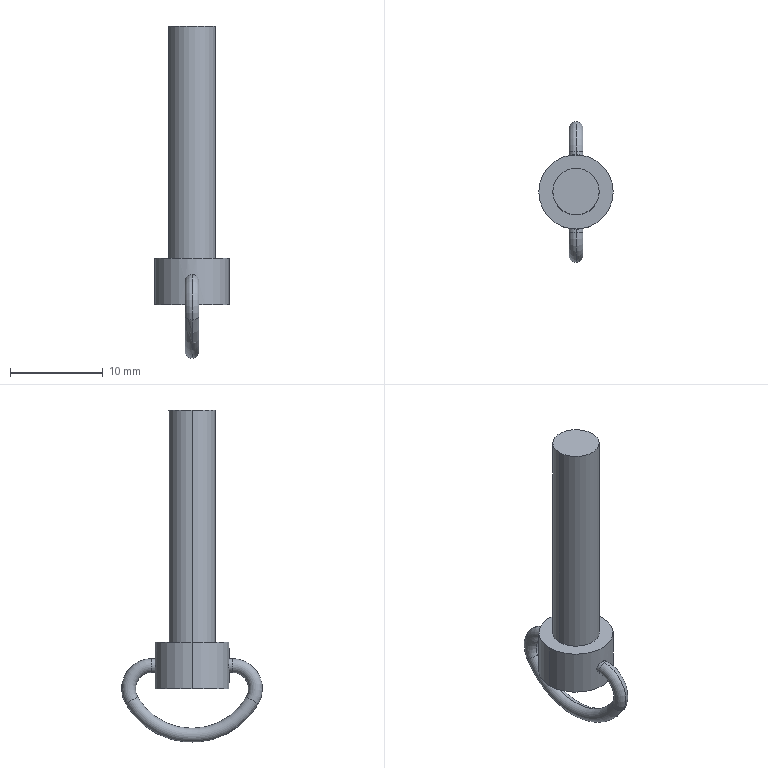Part | SolidWorks | features Extrusion 1, ICE 1, Sweep 1 | 1 solid | 17 faces | box 8 x 15.16 x 35.75 mm | volume 789.697 mm3 | cylinder 8 | torus 6 | plane 3 | commonest cylinder face diameters 1.5 x4 5 x2 8 x2
STEP:
#1=CARTESIAN_POINT('',(0.,4.33,1.75));
#2=VERTEX_POINT('',#1);
#3=CARTESIAN_POINT('',(0.,4.33,3.25));
#4=VERTEX_POINT('',#3);
#5=CARTESIAN_POINT('',(0.,4.33,2.5));
#6=DIRECTION('',(0.,1.,0.));
#7=DIRECTION('',(0.,0.,1.));
#8=AXIS2_PLACEMENT_3D('',#5,#6,#7);
#9=CIRCLE('',#8,0.75);
#10=EDGE_CURVE('',#2,#4,#9,.T.);
#11=ORIENTED_EDGE('',*,*,#10,.T.);
#12=CARTESIAN_POINT('',(0.,7.145,-1.625));
#13=VERTEX_POINT('',#12);
#14=CARTESIAN_POINT('',(0.,4.33,0.));
#15=DIRECTION('',(-1.,0.,0.));
#16=DIRECTION('',(0.,0.,1.));
#17=AXIS2_PLACEMENT_3D('',#14,#15,#16);
#18=CIRCLE('',#17,3.25);
#19=EDGE_CURVE('',#4,#13,#18,.T.);
#20=ORIENTED_EDGE('',*,*,#19,.T.);
#21=CARTESIAN_POINT('',(0.,5.846,-0.875));
#22=VERTEX_POINT('',#21);
#23=CARTESIAN_POINT('',(0.,6.495,-1.25));
#24=DIRECTION('',(0.,-0.5,-0.866));
#25=DIRECTION('',(0.,0.866,-0.5));
#26=AXIS2_PLACEMENT_3D('',#23,#24,#25);
#27=CIRCLE('',#26,0.75);
#28=EDGE_CURVE('',#22,#13,#27,.T.);
#29=ORIENTED_EDGE('',*,*,#28,.F.);
#30=CARTESIAN_POINT('',(0.,4.33,0.));
#31=DIRECTION('',(-1.,0.,0.));
#32=DIRECTION('',(0.,0.,1.));
#33=AXIS2_PLACEMENT_3D('',#30,#31,#32);
#34=CIRCLE('',#33,1.75);
#35=EDGE_CURVE('',#2,#22,#34,.T.);
#36=ORIENTED_EDGE('',*,*,#35,.F.);
#37=EDGE_LOOP('',(#11,#20,#29,#36));
#38=FACE_OUTER_BOUND('',#37,.T.);
#39=CARTESIAN_POINT('',(0.,4.33,0.));
#40=DIRECTION('',(-1.,0.,0.));
#41=DIRECTION('',(0.,0.,1.));
#42=AXIS2_PLACEMENT_3D('',#39,#40,#41);
#43=TOROIDAL_SURFACE('',#42,2.5,0.75);
#44=ADVANCED_FACE('',(#38),#43,.T.);
#45=ORIENTED_EDGE('',*,*,#28,.T.);
#46=CARTESIAN_POINT('',(0.,-7.145,-1.625));
#47=VERTEX_POINT('',#46);
#48=CARTESIAN_POINT('',(0.,0.,2.5));
#49=DIRECTION('',(-1.,0.,0.));
#50=DIRECTION('',(0.,0.,1.));
#51=AXIS2_PLACEMENT_3D('',#48,#49,#50);
#52=CIRCLE('',#51,8.25);
#53=EDGE_CURVE('',#13,#47,#52,.T.);
#54=ORIENTED_EDGE('',*,*,#53,.T.);
#55=CARTESIAN_POINT('',(0.,-5.846,-0.875));
#56=VERTEX_POINT('',#55);
#57=CARTESIAN_POINT('',(0.,-6.495,-1.25));
#58=DIRECTION('',(0.,-0.5,0.866));
#59=DIRECTION('',(0.,-0.866,-0.5));
#60=AXIS2_PLACEMENT_3D('',#57,#58,#59);
#61=CIRCLE('',#60,0.75);
#62=EDGE_CURVE('',#56,#47,#61,.T.);
#63=ORIENTED_EDGE('',*,*,#62,.F.);
#64=CARTESIAN_POINT('',(0.,0.,2.5));
#65=DIRECTION('',(-1.,0.,0.));
#66=DIRECTION('',(0.,0.,1.));
#67=AXIS2_PLACEMENT_3D('',#64,#65,#66);
#68=CIRCLE('',#67,6.75);
#69=EDGE_CURVE('',#22,#56,#68,.T.);
#70=ORIENTED_EDGE('',*,*,#69,.F.);
#71=EDGE_LOOP('',(#45,#54,#63,#70));
#72=FACE_OUTER_BOUND('',#71,.T.);
#73=CARTESIAN_POINT('',(0.,0.,2.5));
#74=DIRECTION('',(-1.,0.,0.));
#75=DIRECTION('',(0.,0.,1.));
#76=AXIS2_PLACEMENT_3D('',#73,#74,#75);
#77=TOROIDAL_SURFACE('',#76,7.5,0.75);
#78=ADVANCED_FACE('',(#72),#77,.T.);
#79=ORIENTED_EDGE('',*,*,#62,.T.);
#80=CARTESIAN_POINT('',(0.,-4.33,3.25));
#81=VERTEX_POINT('',#80);
#82=CARTESIAN_POINT('',(0.,-4.33,0.));
#83=DIRECTION('',(-1.,0.,0.));
#84=DIRECTION('',(0.,0.,1.));
#85=AXIS2_PLACEMENT_3D('',#82,#83,#84);
#86=CIRCLE('',#85,3.25);
#87=EDGE_CURVE('',#47,#81,#86,.T.);
#88=ORIENTED_EDGE('',*,*,#87,.T.);
#89=CARTESIAN_POINT('',(0.,-4.33,1.75));
#90=VERTEX_POINT('',#89);
#91=CARTESIAN_POINT('',(0.,-4.33,2.5));
#92=DIRECTION('',(0.,1.,0.));
#93=DIRECTION('',(0.,0.,1.));
#94=AXIS2_PLACEMENT_3D('',#91,#92,#93);
#95=CIRCLE('',#94,0.75);
#96=EDGE_CURVE('',#90,#81,#95,.T.);
#97=ORIENTED_EDGE('',*,*,#96,.F.);
#98=CARTESIAN_POINT('',(0.,-4.33,0.));
#99=DIRECTION('',(-1.,0.,0.));
#100=DIRECTION('',(0.,0.,1.));
#101=AXIS2_PLACEMENT_3D('',#98,#99,#100);
#102=CIRCLE('',#101,1.75);
#103=EDGE_CURVE('',#56,#90,#102,.T.);
#104=ORIENTED_EDGE('',*,*,#103,.F.);
#105=EDGE_LOOP('',(#79,#88,#97,#104));
#106=FACE_OUTER_BOUND('',#105,.T.);
#107=CARTESIAN_POINT('',(0.,-4.33,0.));
#108=DIRECTION('',(-1.,0.,0.));
#109=DIRECTION('',(0.,0.,1.));
#110=AXIS2_PLACEMENT_3D('',#107,#108,#109);
#111=TOROIDAL_SURFACE('',#110,2.5,0.75);
#112=ADVANCED_FACE('',(#106),#111,.T.);
#113=CARTESIAN_POINT('',(0.,-4.,1.75));
#114=VERTEX_POINT('',#113);
#115=CARTESIAN_POINT('',(0.,-4.,3.25));
#116=VERTEX_POINT('',#115);
#117=CARTESIAN_POINT('',(0.,-4.,1.75));
#118=CARTESIAN_POINT('',(0.09935,-4.,1.75));
#119=CARTESIAN_POINT('',(0.1968,-3.996,1.77));
#120=CARTESIAN_POINT('',(0.3784,-3.983,1.845));
#121=CARTESIAN_POINT('',(0.4614,-3.974,1.901));
#122=CARTESIAN_POINT('',(0.6685,-3.946,2.108));
#123=CARTESIAN_POINT('',(0.7499,-3.929,2.304));
#124=CARTESIAN_POINT('',(0.75,-3.929,2.598));
#125=CARTESIAN_POINT('',(0.7305,-3.933,2.696));
#126=CARTESIAN_POINT('',(0.6552,-3.946,2.878));
#127=CARTESIAN_POINT('',(0.6001,-3.955,2.961));
#128=CARTESIAN_POINT('',(0.4605,-3.974,3.1));
#129=CARTESIAN_POINT('',(0.378,-3.983,3.155));
#130=CARTESIAN_POINT('',(0.1966,-3.996,3.23));
#131=CARTESIAN_POINT('',(0.09801,-4.,3.25));
#132=CARTESIAN_POINT('',(0.,-4.,3.25));
#133=B_SPLINE_CURVE_WITH_KNOTS('',3,(#117,#118,#119,#120,#121,#122,#123,#124,#125,#126,#127,#128,#129,#130,#131,#132),.UNSPECIFIED.,.F.,.F.,(4,2,2,2,2,2,2,4),(0.,0.0002938,0.0005875,0.001175,0.001469,0.001763,0.002056,0.00235),.UNSPECIFIED.);
#134=EDGE_CURVE('',#114,#116,#133,.T.);
#135=ORIENTED_EDGE('',*,*,#134,.T.);
#136=CARTESIAN_POINT('',(0.,4.33,3.25));
#137=DIRECTION('',(0.,-1.,0.));
#138=VECTOR('',#137,1000.);
#139=LINE('',#136,#138);
#140=EDGE_CURVE('',#116,#81,#139,.T.);
#141=ORIENTED_EDGE('',*,*,#140,.T.);
#142=CARTESIAN_POINT('',(0.,-4.33,2.5));
#143=DIRECTION('',(0.,1.,0.));
#144=DIRECTION('',(0.,0.,1.));
#145=AXIS2_PLACEMENT_3D('',#142,#143,#144);
#146=CIRCLE('',#145,0.75);
#147=EDGE_CURVE('',#81,#90,#146,.T.);
#148=ORIENTED_EDGE('',*,*,#147,.T.);
#149=CARTESIAN_POINT('',(0.,4.33,1.75));
#150=DIRECTION('',(0.,-1.,0.));
#151=VECTOR('',#150,1000.);
#152=LINE('',#149,#151);
#153=EDGE_CURVE('',#114,#90,#152,.T.);
#154=ORIENTED_EDGE('',*,*,#153,.F.);
#155=EDGE_LOOP('',(#135,#141,#148,#154));
#156=FACE_OUTER_BOUND('',#155,.T.);
#157=CARTESIAN_POINT('',(0.,4.33,2.5));
#158=DIRECTION('',(0.,-1.,0.));
#159=DIRECTION('',(0.,0.,-1.));
#160=AXIS2_PLACEMENT_3D('',#157,#158,#159);
#161=CYLINDRICAL_SURFACE('',#160,0.75);
#162=ADVANCED_FACE('',(#156),#161,.T.);
#163=CARTESIAN_POINT('',(0.,4.33,2.5));
#164=DIRECTION('',(0.,1.,0.));
#165=DIRECTION('',(0.,0.,1.));
#166=AXIS2_PLACEMENT_3D('',#163,#164,#165);
#167=CIRCLE('',#166,0.75);
#168=EDGE_CURVE('',#4,#2,#167,.T.);
#169=ORIENTED_EDGE('',*,*,#168,.F.);
#170=CARTESIAN_POINT('',(0.,4.,3.25));
#171=VERTEX_POINT('',#170);
#172=CARTESIAN_POINT('',(0.,4.33,3.25));
#173=DIRECTION('',(0.,-1.,0.));
#174=VECTOR('',#173,1000.);
#175=LINE('',#172,#174);
#176=EDGE_CURVE('',#4,#171,#175,.T.);
#177=ORIENTED_EDGE('',*,*,#176,.T.);
#178=CARTESIAN_POINT('',(0.,4.,1.75));
#179=VERTEX_POINT('',#178);
#180=CARTESIAN_POINT('',(0.,4.,3.25));
#181=CARTESIAN_POINT('',(0.196,4.,3.25));
#182=CARTESIAN_POINT('',(0.3917,3.983,3.169));
#183=CARTESIAN_POINT('',(0.6684,3.946,2.892));
#184=CARTESIAN_POINT('',(0.7499,3.929,2.699));
#185=CARTESIAN_POINT('',(0.7501,3.929,2.401));
#186=CARTESIAN_POINT('',(0.7304,3.933,2.304));
#187=CARTESIAN_POINT('',(0.6553,3.946,2.122));
#188=CARTESIAN_POINT('',(0.5996,3.955,2.039));
#189=CARTESIAN_POINT('',(0.3928,3.983,1.832));
#190=CARTESIAN_POINT('',(0.1986,4.,1.75));
#191=CARTESIAN_POINT('',(0.,4.,1.75));
#192=B_SPLINE_CURVE_WITH_KNOTS('',3,(#180,#181,#182,#183,#184,#185,#186,#187,#188,#189,#190,#191),.UNSPECIFIED.,.F.,.F.,(4,2,2,2,2,4),(0.00235,0.002937,0.003525,0.003818,0.004112,0.004699),.UNSPECIFIED.);
#193=EDGE_CURVE('',#171,#179,#192,.T.);
#194=ORIENTED_EDGE('',*,*,#193,.T.);
#195=CARTESIAN_POINT('',(0.,4.33,1.75));
#196=DIRECTION('',(0.,-1.,0.));
#197=VECTOR('',#196,1000.);
#198=LINE('',#195,#197);
#199=EDGE_CURVE('',#2,#179,#198,.T.);
#200=ORIENTED_EDGE('',*,*,#199,.F.);
#201=EDGE_LOOP('',(#169,#177,#194,#200));
#202=FACE_OUTER_BOUND('',#201,.T.);
#203=CARTESIAN_POINT('',(0.,4.33,2.5));
#204=DIRECTION('',(0.,-1.,0.));
#205=DIRECTION('',(0.,0.,-1.));
#206=AXIS2_PLACEMENT_3D('',#203,#204,#205);
#207=CYLINDRICAL_SURFACE('',#206,0.75);
#208=ADVANCED_FACE('',(#202),#207,.T.);
#209=CARTESIAN_POINT('',(2.5,0.,30.));
#210=VERTEX_POINT('',#209);
#211=CARTESIAN_POINT('',(-2.5,0.,30.));
#212=VERTEX_POINT('',#211);
#213=CARTESIAN_POINT('',(0.,0.,30.));
#214=DIRECTION('',(0.,0.,1.));
#215=DIRECTION('',(1.,0.,0.));
#216=AXIS2_PLACEMENT_3D('',#213,#214,#215);
#217=CIRCLE('',#216,2.5);
#218=EDGE_CURVE('',#210,#212,#217,.T.);
#219=ORIENTED_EDGE('',*,*,#218,.F.);
#220=CARTESIAN_POINT('',(2.5,0.,5.));
#221=VERTEX_POINT('',#220);
#222=CARTESIAN_POINT('',(2.5,0.,30.));
#223=DIRECTION('',(0.,0.,-1.));
#224=VECTOR('',#223,1000.);
#225=LINE('',#222,#224);
#226=EDGE_CURVE('',#210,#221,#225,.T.);
#227=ORIENTED_EDGE('',*,*,#226,.T.);
#228=CARTESIAN_POINT('',(-2.5,0.,5.));
#229=VERTEX_POINT('',#228);
#230=CARTESIAN_POINT('',(0.,0.,5.));
#231=DIRECTION('',(0.,0.,1.));
#232=DIRECTION('',(1.,0.,0.));
#233=AXIS2_PLACEMENT_3D('',#230,#231,#232);
#234=CIRCLE('',#233,2.5);
#235=EDGE_CURVE('',#221,#229,#234,.T.);
#236=ORIENTED_EDGE('',*,*,#235,.T.);
#237=CARTESIAN_POINT('',(-2.5,0.,30.));
#238=DIRECTION('',(0.,0.,-1.));
#239=VECTOR('',#238,1000.);
#240=LINE('',#237,#239);
#241=EDGE_CURVE('',#212,#229,#240,.T.);
#242=ORIENTED_EDGE('',*,*,#241,.F.);
#243=EDGE_LOOP('',(#219,#227,#236,#242));
#244=FACE_OUTER_BOUND('',#243,.T.);
#245=CARTESIAN_POINT('',(0.,0.,30.));
#246=DIRECTION('',(0.,0.,-1.));
#247=DIRECTION('',(-1.,0.,0.));
#248=AXIS2_PLACEMENT_3D('',#245,#246,#247);
#249=CYLINDRICAL_SURFACE('',#248,2.5);
#250=ADVANCED_FACE('',(#244),#249,.T.);
#251=CARTESIAN_POINT('',(0.,4.,1.75));
#252=CARTESIAN_POINT('',(-0.09935,4.,1.75));
#253=CARTESIAN_POINT('',(-0.1968,3.996,1.77));
#254=CARTESIAN_POINT('',(-0.3784,3.983,1.845));
#255=CARTESIAN_POINT('',(-0.4614,3.974,1.901));
#256=CARTESIAN_POINT('',(-0.6685,3.946,2.108));
#257=CARTESIAN_POINT('',(-0.7499,3.929,2.304));
#258=CARTESIAN_POINT('',(-0.75,3.929,2.598));
#259=CARTESIAN_POINT('',(-0.7305,3.933,2.696));
#260=CARTESIAN_POINT('',(-0.6552,3.946,2.878));
#261=CARTESIAN_POINT('',(-0.6001,3.955,2.961));
#262=CARTESIAN_POINT('',(-0.4605,3.974,3.1));
#263=CARTESIAN_POINT('',(-0.378,3.983,3.155));
#264=CARTESIAN_POINT('',(-0.1966,3.996,3.23));
#265=CARTESIAN_POINT('',(-0.09801,4.,3.25));
#266=CARTESIAN_POINT('',(0.,4.,3.25));
#267=B_SPLINE_CURVE_WITH_KNOTS('',3,(#251,#252,#253,#254,#255,#256,#257,#258,#259,#260,#261,#262,#263,#264,#265,#266),.UNSPECIFIED.,.F.,.F.,(4,2,2,2,2,2,2,4),(0.,0.0002938,0.0005875,0.001175,0.001469,0.001763,0.002056,0.00235),.UNSPECIFIED.);
#268=EDGE_CURVE('',#179,#171,#267,.T.);
#269=ORIENTED_EDGE('',*,*,#268,.F.);
#270=ORIENTED_EDGE('',*,*,#193,.F.);
#271=EDGE_LOOP('',(#269,#270));
#272=FACE_BOUND('',#271,.T.);
#273=CARTESIAN_POINT('',(4.,0.,5.));
#274=VERTEX_POINT('',#273);
#275=CARTESIAN_POINT('',(-4.,0.,5.));
#276=VERTEX_POINT('',#275);
#277=CARTESIAN_POINT('',(0.,0.,5.));
#278=DIRECTION('',(0.,0.,1.));
#279=DIRECTION('',(1.,0.,0.));
#280=AXIS2_PLACEMENT_3D('',#277,#278,#279);
#281=CIRCLE('',#280,4.);
#282=EDGE_CURVE('',#274,#276,#281,.T.);
#283=ORIENTED_EDGE('',*,*,#282,.F.);
#284=CARTESIAN_POINT('',(4.,0.,0.));
#285=VERTEX_POINT('',#284);
#286=CARTESIAN_POINT('',(4.,0.,5.));
#287=DIRECTION('',(0.,0.,-1.));
#288=VECTOR('',#287,1000.);
#289=LINE('',#286,#288);
#290=EDGE_CURVE('',#274,#285,#289,.T.);
#291=ORIENTED_EDGE('',*,*,#290,.T.);
#292=CARTESIAN_POINT('',(-4.,0.,0.));
#293=VERTEX_POINT('',#292);
#294=CARTESIAN_POINT('',(0.,0.,0.));
#295=DIRECTION('',(0.,0.,1.));
#296=DIRECTION('',(1.,0.,0.));
#297=AXIS2_PLACEMENT_3D('',#294,#295,#296);
#298=CIRCLE('',#297,4.);
#299=EDGE_CURVE('',#285,#293,#298,.T.);
#300=ORIENTED_EDGE('',*,*,#299,.T.);
#301=CARTESIAN_POINT('',(-4.,0.,5.));
#302=DIRECTION('',(0.,0.,-1.));
#303=VECTOR('',#302,1000.);
#304=LINE('',#301,#303);
#305=EDGE_CURVE('',#276,#293,#304,.T.);
#306=ORIENTED_EDGE('',*,*,#305,.F.);
#307=EDGE_LOOP('',(#283,#291,#300,#306));
#308=FACE_OUTER_BOUND('',#307,.T.);
#309=CARTESIAN_POINT('',(0.,0.,5.));
#310=DIRECTION('',(0.,0.,-1.));
#311=DIRECTION('',(-1.,0.,0.));
#312=AXIS2_PLACEMENT_3D('',#309,#310,#311);
#313=CYLINDRICAL_SURFACE('',#312,4.);
#314=ADVANCED_FACE('',(#272,#308),#313,.T.);
#315=ORIENTED_EDGE('',*,*,#290,.F.);
#316=CARTESIAN_POINT('',(0.,0.,5.));
#317=DIRECTION('',(0.,0.,1.));
#318=DIRECTION('',(1.,0.,0.));
#319=AXIS2_PLACEMENT_3D('',#316,#317,#318);
#320=CIRCLE('',#319,4.);
#321=EDGE_CURVE('',#276,#274,#320,.T.);
#322=ORIENTED_EDGE('',*,*,#321,.F.);
#323=ORIENTED_EDGE('',*,*,#305,.T.);
#324=CARTESIAN_POINT('',(0.,0.,0.));
#325=DIRECTION('',(0.,0.,1.));
#326=DIRECTION('',(1.,0.,0.));
#327=AXIS2_PLACEMENT_3D('',#324,#325,#326);
#328=CIRCLE('',#327,4.);
#329=EDGE_CURVE('',#293,#285,#328,.T.);
#330=ORIENTED_EDGE('',*,*,#329,.T.);
#331=EDGE_LOOP('',(#315,#322,#323,#330));
#332=FACE_OUTER_BOUND('',#331,.T.);
#333=ORIENTED_EDGE('',*,*,#134,.F.);
#334=CARTESIAN_POINT('',(0.,-4.,3.25));
#335=CARTESIAN_POINT('',(-0.196,-4.,3.25));
#336=CARTESIAN_POINT('',(-0.3917,-3.983,3.169));
#337=CARTESIAN_POINT('',(-0.6684,-3.946,2.892));
#338=CARTESIAN_POINT('',(-0.7499,-3.929,2.699));
#339=CARTESIAN_POINT('',(-0.7501,-3.929,2.401));
#340=CARTESIAN_POINT('',(-0.7304,-3.933,2.304));
#341=CARTESIAN_POINT('',(-0.6553,-3.946,2.122));
#342=CARTESIAN_POINT('',(-0.5996,-3.955,2.039));
#343=CARTESIAN_POINT('',(-0.3928,-3.983,1.832));
#344=CARTESIAN_POINT('',(-0.1986,-4.,1.75));
#345=CARTESIAN_POINT('',(0.,-4.,1.75));
#346=B_SPLINE_CURVE_WITH_KNOTS('',3,(#334,#335,#336,#337,#338,#339,#340,#341,#342,#343,#344,#345),.UNSPECIFIED.,.F.,.F.,(4,2,2,2,2,4),(0.00235,0.002937,0.003525,0.003818,0.004112,0.004699),.UNSPECIFIED.);
#347=EDGE_CURVE('',#116,#114,#346,.T.);
#348=ORIENTED_EDGE('',*,*,#347,.F.);
#349=EDGE_LOOP('',(#333,#348));
#350=FACE_BOUND('',#349,.T.);
#351=CARTESIAN_POINT('',(0.,0.,5.));
#352=DIRECTION('',(0.,0.,-1.));
#353=DIRECTION('',(-1.,0.,0.));
#354=AXIS2_PLACEMENT_3D('',#351,#352,#353);
#355=CYLINDRICAL_SURFACE('',#354,4.);
#356=ADVANCED_FACE('',(#332,#350),#355,.T.);
#357=ORIENTED_EDGE('',*,*,#321,.T.);
#358=ORIENTED_EDGE('',*,*,#282,.T.);
#359=EDGE_LOOP('',(#357,#358));
#360=FACE_OUTER_BOUND('',#359,.T.);
#361=CARTESIAN_POINT('',(0.,0.,5.));
#362=DIRECTION('',(0.,0.,1.));
#363=DIRECTION('',(1.,0.,0.));
#364=AXIS2_PLACEMENT_3D('',#361,#362,#363);
#365=CIRCLE('',#364,2.5);
#366=EDGE_CURVE('',#229,#221,#365,.T.);
#367=ORIENTED_EDGE('',*,*,#366,.F.);
#368=ORIENTED_EDGE('',*,*,#235,.F.);
#369=EDGE_LOOP('',(#367,#368));
#370=FACE_BOUND('',#369,.T.);
#371=CARTESIAN_POINT('',(0.,0.,5.));
#372=DIRECTION('',(0.,0.,1.));
#373=DIRECTION('',(1.,0.,0.));
#374=AXIS2_PLACEMENT_3D('',#371,#372,#373);
#375=PLANE('',#374);
#376=ADVANCED_FACE('',(#360,#370),#375,.T.);
#377=ORIENTED_EDGE('',*,*,#329,.F.);
#378=ORIENTED_EDGE('',*,*,#299,.F.);
#379=EDGE_LOOP('',(#377,#378));
#380=FACE_OUTER_BOUND('',#379,.T.);
#381=CARTESIAN_POINT('',(0.,0.,0.));
#382=DIRECTION('',(0.,0.,1.));
#383=DIRECTION('',(1.,0.,0.));
#384=AXIS2_PLACEMENT_3D('',#381,#382,#383);
#385=PLANE('',#384);
#386=ADVANCED_FACE('',(#380),#385,.F.);
#387=ORIENTED_EDGE('',*,*,#226,.F.);
#388=CARTESIAN_POINT('',(0.,0.,30.));
#389=DIRECTION('',(0.,0.,1.));
#390=DIRECTION('',(1.,0.,0.));
#391=AXIS2_PLACEMENT_3D('',#388,#389,#390);
#392=CIRCLE('',#391,2.5);
#393=EDGE_CURVE('',#212,#210,#392,.T.);
#394=ORIENTED_EDGE('',*,*,#393,.F.);
#395=ORIENTED_EDGE('',*,*,#241,.T.);
#396=ORIENTED_EDGE('',*,*,#366,.T.);
#397=EDGE_LOOP('',(#387,#394,#395,#396));
#398=FACE_OUTER_BOUND('',#397,.T.);
#399=CARTESIAN_POINT('',(0.,0.,30.));
#400=DIRECTION('',(0.,0.,-1.));
#401=DIRECTION('',(-1.,0.,0.));
#402=AXIS2_PLACEMENT_3D('',#399,#400,#401);
#403=CYLINDRICAL_SURFACE('',#402,2.5);
#404=ADVANCED_FACE('',(#398),#403,.T.);
#405=ORIENTED_EDGE('',*,*,#393,.T.);
#406=ORIENTED_EDGE('',*,*,#218,.T.);
#407=EDGE_LOOP('',(#405,#406));
#408=FACE_OUTER_BOUND('',#407,.T.);
#409=CARTESIAN_POINT('',(0.,0.,30.));
#410=DIRECTION('',(0.,0.,1.));
#411=DIRECTION('',(1.,0.,0.));
#412=AXIS2_PLACEMENT_3D('',#409,#410,#411);
#413=PLANE('',#412);
#414=ADVANCED_FACE('',(#408),#413,.T.);
#415=ORIENTED_EDGE('',*,*,#176,.F.);
#416=ORIENTED_EDGE('',*,*,#10,.F.);
#417=ORIENTED_EDGE('',*,*,#199,.T.);
#418=ORIENTED_EDGE('',*,*,#268,.T.);
#419=EDGE_LOOP('',(#415,#416,#417,#418));
#420=FACE_OUTER_BOUND('',#419,.T.);
#421=CARTESIAN_POINT('',(0.,4.33,2.5));
#422=DIRECTION('',(0.,-1.,0.));
#423=DIRECTION('',(0.,0.,-1.));
#424=AXIS2_PLACEMENT_3D('',#421,#422,#423);
#425=CYLINDRICAL_SURFACE('',#424,0.75);
#426=ADVANCED_FACE('',(#420),#425,.T.);
#427=ORIENTED_EDGE('',*,*,#140,.F.);
#428=ORIENTED_EDGE('',*,*,#347,.T.);
#429=ORIENTED_EDGE('',*,*,#153,.T.);
#430=ORIENTED_EDGE('',*,*,#96,.T.);
#431=EDGE_LOOP('',(#427,#428,#429,#430));
#432=FACE_OUTER_BOUND('',#431,.T.);
#433=CARTESIAN_POINT('',(0.,4.33,2.5));
#434=DIRECTION('',(0.,-1.,0.));
#435=DIRECTION('',(0.,0.,-1.));
#436=AXIS2_PLACEMENT_3D('',#433,#434,#435);
#437=CYLINDRICAL_SURFACE('',#436,0.75);
#438=ADVANCED_FACE('',(#432),#437,.T.);
#439=ORIENTED_EDGE('',*,*,#87,.F.);
#440=CARTESIAN_POINT('',(0.,-6.495,-1.25));
#441=DIRECTION('',(0.,-0.5,0.866));
#442=DIRECTION('',(0.,-0.866,-0.5));
#443=AXIS2_PLACEMENT_3D('',#440,#441,#442);
#444=CIRCLE('',#443,0.75);
#445=EDGE_CURVE('',#47,#56,#444,.T.);
#446=ORIENTED_EDGE('',*,*,#445,.T.);
#447=ORIENTED_EDGE('',*,*,#103,.T.);
#448=ORIENTED_EDGE('',*,*,#147,.F.);
#449=EDGE_LOOP('',(#439,#446,#447,#448));
#450=FACE_OUTER_BOUND('',#449,.T.);
#451=CARTESIAN_POINT('',(0.,-4.33,0.));
#452=DIRECTION('',(-1.,0.,0.));
#453=DIRECTION('',(0.,0.,1.));
#454=AXIS2_PLACEMENT_3D('',#451,#452,#453);
#455=TOROIDAL_SURFACE('',#454,2.5,0.75);
#456=ADVANCED_FACE('',(#450),#455,.T.);
#457=ORIENTED_EDGE('',*,*,#53,.F.);
#458=CARTESIAN_POINT('',(0.,6.495,-1.25));
#459=DIRECTION('',(0.,-0.5,-0.866));
#460=DIRECTION('',(0.,0.866,-0.5));
#461=AXIS2_PLACEMENT_3D('',#458,#459,#460);
#462=CIRCLE('',#461,0.75);
#463=EDGE_CURVE('',#13,#22,#462,.T.);
#464=ORIENTED_EDGE('',*,*,#463,.T.);
#465=ORIENTED_EDGE('',*,*,#69,.T.);
#466=ORIENTED_EDGE('',*,*,#445,.F.);
#467=EDGE_LOOP('',(#457,#464,#465,#466));
#468=FACE_OUTER_BOUND('',#467,.T.);
#469=CARTESIAN_POINT('',(0.,0.,2.5));
#470=DIRECTION('',(-1.,0.,0.));
#471=DIRECTION('',(0.,0.,1.));
#472=AXIS2_PLACEMENT_3D('',#469,#470,#471);
#473=TOROIDAL_SURFACE('',#472,7.5,0.75);
#474=ADVANCED_FACE('',(#468),#473,.T.);
#475=ORIENTED_EDGE('',*,*,#19,.F.);
#476=ORIENTED_EDGE('',*,*,#168,.T.);
#477=ORIENTED_EDGE('',*,*,#35,.T.);
#478=ORIENTED_EDGE('',*,*,#463,.F.);
#479=EDGE_LOOP('',(#475,#476,#477,#478));
#480=FACE_OUTER_BOUND('',#479,.T.);
#481=CARTESIAN_POINT('',(0.,4.33,0.));
#482=DIRECTION('',(-1.,0.,0.));
#483=DIRECTION('',(0.,0.,1.));
#484=AXIS2_PLACEMENT_3D('',#481,#482,#483);
#485=TOROIDAL_SURFACE('',#484,2.5,0.75);
#486=ADVANCED_FACE('',(#480),#485,.T.);
#487=CLOSED_SHELL('',(#44,#78,#112,#162,#208,#250,#314,#356,#376,#386,#404,#414,#426,#438,#456,#474,#486));
#488=MANIFOLD_SOLID_BREP('',#487);
#489=CARTESIAN_POINT('',(0.,0.,0.));
#490=DIRECTION('',(0.,0.,1.));
#491=DIRECTION('',(1.,0.,0.));
#492=AXIS2_PLACEMENT_3D('',#489,#490,#491);
#493=(LENGTH_UNIT()NAMED_UNIT(*)SI_UNIT(.MILLI.,.METRE.));
#494=UNCERTAINTY_MEASURE_WITH_UNIT(LENGTH_MEASURE(0.00001),#493,'','');
#495=(NAMED_UNIT(*)PLANE_ANGLE_UNIT()SI_UNIT($,.RADIAN.));
#496=(NAMED_UNIT(*)SI_UNIT($,.STERADIAN.)SOLID_ANGLE_UNIT());
#497=(GEOMETRIC_REPRESENTATION_CONTEXT(3)GLOBAL_UNCERTAINTY_ASSIGNED_CONTEXT((#494))GLOBAL_UNIT_ASSIGNED_CONTEXT((#493,#495,#496))REPRESENTATION_CONTEXT('',''));
#498=ADVANCED_BREP_SHAPE_REPRESENTATION('',(#488,#492),#497);